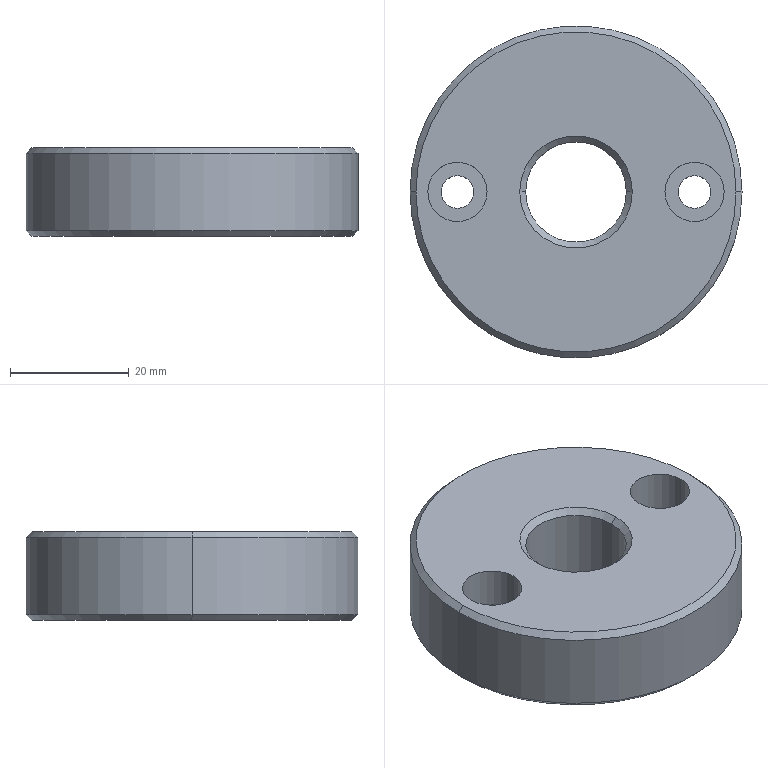Part | SolidWorks | features HoleWzd 2, Chamfer 1, Extrusion 1 | 1 solid | 24 faces | box 56 x 56 x 15 mm | volume 31831 mm3 | cylinder 12 | cone 8 | plane 4 | commonest cylinder face diameters 5.5 x4 10 x4 17 x2 56 x2
STEP:
#1=CARTESIAN_POINT('',(27.,0.,15.));
#2=VERTEX_POINT('',#1);
#3=CARTESIAN_POINT('',(-27.,0.,15.));
#4=VERTEX_POINT('',#3);
#5=CARTESIAN_POINT('',(0.,0.,15.));
#6=DIRECTION('',(0.,0.,1.));
#7=DIRECTION('',(1.,0.,0.));
#8=AXIS2_PLACEMENT_3D('',#5,#6,#7);
#9=CIRCLE('',#8,27.);
#10=EDGE_CURVE('',#2,#4,#9,.T.);
#11=ORIENTED_EDGE('',*,*,#10,.F.);
#12=CARTESIAN_POINT('',(28.,0.,14.));
#13=VERTEX_POINT('',#12);
#14=CARTESIAN_POINT('',(27.,0.,15.));
#15=DIRECTION('',(0.7071,0.,-0.7071));
#16=VECTOR('',#15,1000.);
#17=LINE('',#14,#16);
#18=EDGE_CURVE('',#2,#13,#17,.T.);
#19=ORIENTED_EDGE('',*,*,#18,.T.);
#20=CARTESIAN_POINT('',(-28.,0.,14.));
#21=VERTEX_POINT('',#20);
#22=CARTESIAN_POINT('',(0.,0.,14.));
#23=DIRECTION('',(0.,0.,-1.));
#24=DIRECTION('',(1.,0.,0.));
#25=AXIS2_PLACEMENT_3D('',#22,#23,#24);
#26=CIRCLE('',#25,28.);
#27=EDGE_CURVE('',#21,#13,#26,.T.);
#28=ORIENTED_EDGE('',*,*,#27,.F.);
#29=CARTESIAN_POINT('',(-27.,0.,15.));
#30=DIRECTION('',(-0.7071,0.,-0.7071));
#31=VECTOR('',#30,1000.);
#32=LINE('',#29,#31);
#33=EDGE_CURVE('',#4,#21,#32,.T.);
#34=ORIENTED_EDGE('',*,*,#33,.F.);
#35=EDGE_LOOP('',(#11,#19,#28,#34));
#36=FACE_OUTER_BOUND('',#35,.T.);
#37=CARTESIAN_POINT('',(0.,0.,15.));
#38=DIRECTION('',(0.,0.,-1.));
#39=DIRECTION('',(-1.,0.,0.));
#40=AXIS2_PLACEMENT_3D('',#37,#38,#39);
#41=CONICAL_SURFACE('',#40,27.,0.7854);
#42=ADVANCED_FACE('',(#36),#41,.T.);
#43=CARTESIAN_POINT('',(-27.,0.,0.));
#44=VERTEX_POINT('',#43);
#45=CARTESIAN_POINT('',(27.,0.,0.));
#46=VERTEX_POINT('',#45);
#47=CARTESIAN_POINT('',(0.,0.,0.));
#48=DIRECTION('',(0.,0.,-1.));
#49=DIRECTION('',(1.,0.,0.));
#50=AXIS2_PLACEMENT_3D('',#47,#48,#49);
#51=CIRCLE('',#50,27.);
#52=EDGE_CURVE('',#44,#46,#51,.T.);
#53=ORIENTED_EDGE('',*,*,#52,.F.);
#54=CARTESIAN_POINT('',(-28.,0.,1.));
#55=VERTEX_POINT('',#54);
#56=CARTESIAN_POINT('',(-28.,0.,1.));
#57=DIRECTION('',(-0.7071,0.,0.7071));
#58=VECTOR('',#57,1000.);
#59=LINE('',#56,#58);
#60=EDGE_CURVE('',#44,#55,#59,.T.);
#61=ORIENTED_EDGE('',*,*,#60,.T.);
#62=CARTESIAN_POINT('',(28.,0.,1.));
#63=VERTEX_POINT('',#62);
#64=CARTESIAN_POINT('',(0.,0.,1.));
#65=DIRECTION('',(0.,0.,1.));
#66=DIRECTION('',(1.,0.,0.));
#67=AXIS2_PLACEMENT_3D('',#64,#65,#66);
#68=CIRCLE('',#67,28.);
#69=EDGE_CURVE('',#63,#55,#68,.T.);
#70=ORIENTED_EDGE('',*,*,#69,.F.);
#71=CARTESIAN_POINT('',(28.,0.,1.));
#72=DIRECTION('',(0.7071,0.,0.7071));
#73=VECTOR('',#72,1000.);
#74=LINE('',#71,#73);
#75=EDGE_CURVE('',#46,#63,#74,.T.);
#76=ORIENTED_EDGE('',*,*,#75,.F.);
#77=EDGE_LOOP('',(#53,#61,#70,#76));
#78=FACE_OUTER_BOUND('',#77,.T.);
#79=CARTESIAN_POINT('',(0.,0.,1.));
#80=DIRECTION('',(0.,0.,1.));
#81=DIRECTION('',(1.,0.,0.));
#82=AXIS2_PLACEMENT_3D('',#79,#80,#81);
#83=CONICAL_SURFACE('',#82,28.,0.7854);
#84=ADVANCED_FACE('',(#78),#83,.T.);
#85=CARTESIAN_POINT('',(8.5,0.,1.));
#86=VERTEX_POINT('',#85);
#87=CARTESIAN_POINT('',(-8.5,0.,1.));
#88=VERTEX_POINT('',#87);
#89=CARTESIAN_POINT('',(0.,0.,1.));
#90=DIRECTION('',(0.,0.,-1.));
#91=DIRECTION('',(1.,0.,0.));
#92=AXIS2_PLACEMENT_3D('',#89,#90,#91);
#93=CIRCLE('',#92,8.5);
#94=EDGE_CURVE('',#86,#88,#93,.T.);
#95=ORIENTED_EDGE('',*,*,#94,.F.);
#96=CARTESIAN_POINT('',(9.5,0.,0.));
#97=VERTEX_POINT('',#96);
#98=CARTESIAN_POINT('',(9.5,0.,0.));
#99=DIRECTION('',(0.7071,0.,-0.7071));
#100=VECTOR('',#99,1000.);
#101=LINE('',#98,#100);
#102=EDGE_CURVE('',#86,#97,#101,.T.);
#103=ORIENTED_EDGE('',*,*,#102,.T.);
#104=CARTESIAN_POINT('',(-9.5,0.,0.));
#105=VERTEX_POINT('',#104);
#106=CARTESIAN_POINT('',(0.,0.,0.));
#107=DIRECTION('',(0.,0.,1.));
#108=DIRECTION('',(1.,0.,0.));
#109=AXIS2_PLACEMENT_3D('',#106,#107,#108);
#110=CIRCLE('',#109,9.5);
#111=EDGE_CURVE('',#105,#97,#110,.T.);
#112=ORIENTED_EDGE('',*,*,#111,.F.);
#113=CARTESIAN_POINT('',(-9.5,0.,0.));
#114=DIRECTION('',(-0.7071,0.,-0.7071));
#115=VECTOR('',#114,1000.);
#116=LINE('',#113,#115);
#117=EDGE_CURVE('',#88,#105,#116,.T.);
#118=ORIENTED_EDGE('',*,*,#117,.F.);
#119=EDGE_LOOP('',(#95,#103,#112,#118));
#120=FACE_OUTER_BOUND('',#119,.T.);
#121=CARTESIAN_POINT('',(0.,0.,0.));
#122=DIRECTION('',(0.,0.,-1.));
#123=DIRECTION('',(-1.,0.,0.));
#124=AXIS2_PLACEMENT_3D('',#121,#122,#123);
#125=CONICAL_SURFACE('',#124,9.5,0.7854);
#126=ADVANCED_FACE('',(#120),#125,.F.);
#127=CARTESIAN_POINT('',(-8.5,0.,14.));
#128=VERTEX_POINT('',#127);
#129=CARTESIAN_POINT('',(8.5,0.,14.));
#130=VERTEX_POINT('',#129);
#131=CARTESIAN_POINT('',(0.,0.,14.));
#132=DIRECTION('',(0.,0.,1.));
#133=DIRECTION('',(1.,0.,0.));
#134=AXIS2_PLACEMENT_3D('',#131,#132,#133);
#135=CIRCLE('',#134,8.5);
#136=EDGE_CURVE('',#128,#130,#135,.T.);
#137=ORIENTED_EDGE('',*,*,#136,.F.);
#138=CARTESIAN_POINT('',(-9.5,0.,15.));
#139=VERTEX_POINT('',#138);
#140=CARTESIAN_POINT('',(-8.5,0.,14.));
#141=DIRECTION('',(-0.7071,0.,0.7071));
#142=VECTOR('',#141,1000.);
#143=LINE('',#140,#142);
#144=EDGE_CURVE('',#128,#139,#143,.T.);
#145=ORIENTED_EDGE('',*,*,#144,.T.);
#146=CARTESIAN_POINT('',(9.5,0.,15.));
#147=VERTEX_POINT('',#146);
#148=CARTESIAN_POINT('',(0.,0.,15.));
#149=DIRECTION('',(0.,0.,-1.));
#150=DIRECTION('',(1.,0.,0.));
#151=AXIS2_PLACEMENT_3D('',#148,#149,#150);
#152=CIRCLE('',#151,9.5);
#153=EDGE_CURVE('',#147,#139,#152,.T.);
#154=ORIENTED_EDGE('',*,*,#153,.F.);
#155=CARTESIAN_POINT('',(8.5,0.,14.));
#156=DIRECTION('',(0.7071,0.,0.7071));
#157=VECTOR('',#156,1000.);
#158=LINE('',#155,#157);
#159=EDGE_CURVE('',#130,#147,#158,.T.);
#160=ORIENTED_EDGE('',*,*,#159,.F.);
#161=EDGE_LOOP('',(#137,#145,#154,#160));
#162=FACE_OUTER_BOUND('',#161,.T.);
#163=CARTESIAN_POINT('',(0.,0.,14.));
#164=DIRECTION('',(0.,0.,1.));
#165=DIRECTION('',(1.,0.,0.));
#166=AXIS2_PLACEMENT_3D('',#163,#164,#165);
#167=CONICAL_SURFACE('',#166,8.5,0.7854);
#168=ADVANCED_FACE('',(#162),#167,.F.);
#169=CARTESIAN_POINT('',(-25.,0.,8.));
#170=VERTEX_POINT('',#169);
#171=CARTESIAN_POINT('',(-15.,0.,8.));
#172=VERTEX_POINT('',#171);
#173=CARTESIAN_POINT('',(-20.,0.,8.));
#174=DIRECTION('',(0.,0.,1.));
#175=DIRECTION('',(1.,0.,0.));
#176=AXIS2_PLACEMENT_3D('',#173,#174,#175);
#177=CIRCLE('',#176,5.);
#178=EDGE_CURVE('',#170,#172,#177,.T.);
#179=ORIENTED_EDGE('',*,*,#178,.F.);
#180=CARTESIAN_POINT('',(-25.,0.,15.));
#181=VERTEX_POINT('',#180);
#182=CARTESIAN_POINT('',(-25.,0.,15.));
#183=DIRECTION('',(0.,0.,1.));
#184=VECTOR('',#183,1000.);
#185=LINE('',#182,#184);
#186=EDGE_CURVE('',#170,#181,#185,.T.);
#187=ORIENTED_EDGE('',*,*,#186,.T.);
#188=CARTESIAN_POINT('',(-15.,0.,15.));
#189=VERTEX_POINT('',#188);
#190=CARTESIAN_POINT('',(-20.,0.,15.));
#191=DIRECTION('',(0.,0.,1.));
#192=DIRECTION('',(1.,0.,0.));
#193=AXIS2_PLACEMENT_3D('',#190,#191,#192);
#194=CIRCLE('',#193,5.);
#195=EDGE_CURVE('',#181,#189,#194,.T.);
#196=ORIENTED_EDGE('',*,*,#195,.T.);
#197=CARTESIAN_POINT('',(-15.,0.,15.));
#198=DIRECTION('',(0.,0.,1.));
#199=VECTOR('',#198,1000.);
#200=LINE('',#197,#199);
#201=EDGE_CURVE('',#172,#189,#200,.T.);
#202=ORIENTED_EDGE('',*,*,#201,.F.);
#203=EDGE_LOOP('',(#179,#187,#196,#202));
#204=FACE_OUTER_BOUND('',#203,.T.);
#205=CARTESIAN_POINT('',(-20.,0.,15.));
#206=DIRECTION('',(0.,0.,1.));
#207=DIRECTION('',(1.,0.,0.));
#208=AXIS2_PLACEMENT_3D('',#205,#206,#207);
#209=CYLINDRICAL_SURFACE('',#208,5.);
#210=ADVANCED_FACE('',(#204),#209,.F.);
#211=CARTESIAN_POINT('',(-22.75,0.,0.));
#212=VERTEX_POINT('',#211);
#213=CARTESIAN_POINT('',(-17.25,0.,0.));
#214=VERTEX_POINT('',#213);
#215=CARTESIAN_POINT('',(-20.,0.,0.));
#216=DIRECTION('',(0.,0.,1.));
#217=DIRECTION('',(1.,0.,0.));
#218=AXIS2_PLACEMENT_3D('',#215,#216,#217);
#219=CIRCLE('',#218,2.75);
#220=EDGE_CURVE('',#212,#214,#219,.T.);
#221=ORIENTED_EDGE('',*,*,#220,.F.);
#222=CARTESIAN_POINT('',(-22.75,0.,8.));
#223=VERTEX_POINT('',#222);
#224=CARTESIAN_POINT('',(-22.75,0.,15.));
#225=DIRECTION('',(0.,0.,1.));
#226=VECTOR('',#225,1000.);
#227=LINE('',#224,#226);
#228=EDGE_CURVE('',#212,#223,#227,.T.);
#229=ORIENTED_EDGE('',*,*,#228,.T.);
#230=CARTESIAN_POINT('',(-17.25,0.,8.));
#231=VERTEX_POINT('',#230);
#232=CARTESIAN_POINT('',(-20.,0.,8.));
#233=DIRECTION('',(0.,0.,1.));
#234=DIRECTION('',(1.,0.,0.));
#235=AXIS2_PLACEMENT_3D('',#232,#233,#234);
#236=CIRCLE('',#235,2.75);
#237=EDGE_CURVE('',#223,#231,#236,.T.);
#238=ORIENTED_EDGE('',*,*,#237,.T.);
#239=CARTESIAN_POINT('',(-17.25,0.,15.));
#240=DIRECTION('',(0.,0.,1.));
#241=VECTOR('',#240,1000.);
#242=LINE('',#239,#241);
#243=EDGE_CURVE('',#214,#231,#242,.T.);
#244=ORIENTED_EDGE('',*,*,#243,.F.);
#245=EDGE_LOOP('',(#221,#229,#238,#244));
#246=FACE_OUTER_BOUND('',#245,.T.);
#247=CARTESIAN_POINT('',(-20.,0.,15.));
#248=DIRECTION('',(0.,0.,1.));
#249=DIRECTION('',(1.,0.,0.));
#250=AXIS2_PLACEMENT_3D('',#247,#248,#249);
#251=CYLINDRICAL_SURFACE('',#250,2.75);
#252=ADVANCED_FACE('',(#246),#251,.F.);
#253=CARTESIAN_POINT('',(15.,0.,8.));
#254=VERTEX_POINT('',#253);
#255=CARTESIAN_POINT('',(25.,0.,8.));
#256=VERTEX_POINT('',#255);
#257=CARTESIAN_POINT('',(20.,0.,8.));
#258=DIRECTION('',(0.,0.,1.));
#259=DIRECTION('',(1.,0.,0.));
#260=AXIS2_PLACEMENT_3D('',#257,#258,#259);
#261=CIRCLE('',#260,5.);
#262=EDGE_CURVE('',#254,#256,#261,.T.);
#263=ORIENTED_EDGE('',*,*,#262,.F.);
#264=CARTESIAN_POINT('',(15.,0.,15.));
#265=VERTEX_POINT('',#264);
#266=CARTESIAN_POINT('',(15.,0.,15.));
#267=DIRECTION('',(0.,0.,1.));
#268=VECTOR('',#267,1000.);
#269=LINE('',#266,#268);
#270=EDGE_CURVE('',#254,#265,#269,.T.);
#271=ORIENTED_EDGE('',*,*,#270,.T.);
#272=CARTESIAN_POINT('',(25.,0.,15.));
#273=VERTEX_POINT('',#272);
#274=CARTESIAN_POINT('',(20.,0.,15.));
#275=DIRECTION('',(0.,0.,1.));
#276=DIRECTION('',(1.,0.,0.));
#277=AXIS2_PLACEMENT_3D('',#274,#275,#276);
#278=CIRCLE('',#277,5.);
#279=EDGE_CURVE('',#265,#273,#278,.T.);
#280=ORIENTED_EDGE('',*,*,#279,.T.);
#281=CARTESIAN_POINT('',(25.,0.,15.));
#282=DIRECTION('',(0.,0.,1.));
#283=VECTOR('',#282,1000.);
#284=LINE('',#281,#283);
#285=EDGE_CURVE('',#256,#273,#284,.T.);
#286=ORIENTED_EDGE('',*,*,#285,.F.);
#287=EDGE_LOOP('',(#263,#271,#280,#286));
#288=FACE_OUTER_BOUND('',#287,.T.);
#289=CARTESIAN_POINT('',(20.,0.,15.));
#290=DIRECTION('',(0.,0.,1.));
#291=DIRECTION('',(1.,0.,0.));
#292=AXIS2_PLACEMENT_3D('',#289,#290,#291);
#293=CYLINDRICAL_SURFACE('',#292,5.);
#294=ADVANCED_FACE('',(#288),#293,.F.);
#295=CARTESIAN_POINT('',(17.25,0.,0.));
#296=VERTEX_POINT('',#295);
#297=CARTESIAN_POINT('',(22.75,0.,0.));
#298=VERTEX_POINT('',#297);
#299=CARTESIAN_POINT('',(20.,0.,0.));
#300=DIRECTION('',(0.,0.,1.));
#301=DIRECTION('',(1.,0.,0.));
#302=AXIS2_PLACEMENT_3D('',#299,#300,#301);
#303=CIRCLE('',#302,2.75);
#304=EDGE_CURVE('',#296,#298,#303,.T.);
#305=ORIENTED_EDGE('',*,*,#304,.F.);
#306=CARTESIAN_POINT('',(17.25,0.,8.));
#307=VERTEX_POINT('',#306);
#308=CARTESIAN_POINT('',(17.25,0.,15.));
#309=DIRECTION('',(0.,0.,1.));
#310=VECTOR('',#309,1000.);
#311=LINE('',#308,#310);
#312=EDGE_CURVE('',#296,#307,#311,.T.);
#313=ORIENTED_EDGE('',*,*,#312,.T.);
#314=CARTESIAN_POINT('',(22.75,0.,8.));
#315=VERTEX_POINT('',#314);
#316=CARTESIAN_POINT('',(20.,0.,8.));
#317=DIRECTION('',(0.,0.,1.));
#318=DIRECTION('',(1.,0.,0.));
#319=AXIS2_PLACEMENT_3D('',#316,#317,#318);
#320=CIRCLE('',#319,2.75);
#321=EDGE_CURVE('',#307,#315,#320,.T.);
#322=ORIENTED_EDGE('',*,*,#321,.T.);
#323=CARTESIAN_POINT('',(22.75,0.,15.));
#324=DIRECTION('',(0.,0.,1.));
#325=VECTOR('',#324,1000.);
#326=LINE('',#323,#325);
#327=EDGE_CURVE('',#298,#315,#326,.T.);
#328=ORIENTED_EDGE('',*,*,#327,.F.);
#329=EDGE_LOOP('',(#305,#313,#322,#328));
#330=FACE_OUTER_BOUND('',#329,.T.);
#331=CARTESIAN_POINT('',(20.,0.,15.));
#332=DIRECTION('',(0.,0.,1.));
#333=DIRECTION('',(1.,0.,0.));
#334=AXIS2_PLACEMENT_3D('',#331,#332,#333);
#335=CYLINDRICAL_SURFACE('',#334,2.75);
#336=ADVANCED_FACE('',(#330),#335,.F.);
#337=ORIENTED_EDGE('',*,*,#94,.T.);
#338=CARTESIAN_POINT('',(-8.5,0.,15.));
#339=DIRECTION('',(0.,0.,1.));
#340=VECTOR('',#339,1000.);
#341=LINE('',#338,#340);
#342=EDGE_CURVE('',#88,#128,#341,.T.);
#343=ORIENTED_EDGE('',*,*,#342,.T.);
#344=ORIENTED_EDGE('',*,*,#136,.T.);
#345=CARTESIAN_POINT('',(8.5,0.,15.));
#346=DIRECTION('',(0.,0.,1.));
#347=VECTOR('',#346,1000.);
#348=LINE('',#345,#347);
#349=EDGE_CURVE('',#86,#130,#348,.T.);
#350=ORIENTED_EDGE('',*,*,#349,.F.);
#351=EDGE_LOOP('',(#337,#343,#344,#350));
#352=FACE_OUTER_BOUND('',#351,.T.);
#353=CARTESIAN_POINT('',(0.,0.,15.));
#354=DIRECTION('',(0.,0.,1.));
#355=DIRECTION('',(1.,0.,0.));
#356=AXIS2_PLACEMENT_3D('',#353,#354,#355);
#357=CYLINDRICAL_SURFACE('',#356,8.5);
#358=ADVANCED_FACE('',(#352),#357,.F.);
#359=ORIENTED_EDGE('',*,*,#27,.T.);
#360=CARTESIAN_POINT('',(28.,0.,15.));
#361=DIRECTION('',(0.,0.,-1.));
#362=VECTOR('',#361,1000.);
#363=LINE('',#360,#362);
#364=EDGE_CURVE('',#13,#63,#363,.T.);
#365=ORIENTED_EDGE('',*,*,#364,.T.);
#366=ORIENTED_EDGE('',*,*,#69,.T.);
#367=CARTESIAN_POINT('',(-28.,0.,15.));
#368=DIRECTION('',(0.,0.,-1.));
#369=VECTOR('',#368,1000.);
#370=LINE('',#367,#369);
#371=EDGE_CURVE('',#21,#55,#370,.T.);
#372=ORIENTED_EDGE('',*,*,#371,.F.);
#373=EDGE_LOOP('',(#359,#365,#366,#372));
#374=FACE_OUTER_BOUND('',#373,.T.);
#375=CARTESIAN_POINT('',(0.,0.,15.));
#376=DIRECTION('',(0.,0.,-1.));
#377=DIRECTION('',(-1.,0.,0.));
#378=AXIS2_PLACEMENT_3D('',#375,#376,#377);
#379=CYLINDRICAL_SURFACE('',#378,28.);
#380=ADVANCED_FACE('',(#374),#379,.T.);
#381=ORIENTED_EDGE('',*,*,#364,.F.);
#382=CARTESIAN_POINT('',(0.,0.,14.));
#383=DIRECTION('',(0.,0.,-1.));
#384=DIRECTION('',(1.,0.,0.));
#385=AXIS2_PLACEMENT_3D('',#382,#383,#384);
#386=CIRCLE('',#385,28.);
#387=EDGE_CURVE('',#13,#21,#386,.T.);
#388=ORIENTED_EDGE('',*,*,#387,.T.);
#389=ORIENTED_EDGE('',*,*,#371,.T.);
#390=CARTESIAN_POINT('',(0.,0.,1.));
#391=DIRECTION('',(0.,0.,1.));
#392=DIRECTION('',(1.,0.,0.));
#393=AXIS2_PLACEMENT_3D('',#390,#391,#392);
#394=CIRCLE('',#393,28.);
#395=EDGE_CURVE('',#55,#63,#394,.T.);
#396=ORIENTED_EDGE('',*,*,#395,.T.);
#397=EDGE_LOOP('',(#381,#388,#389,#396));
#398=FACE_OUTER_BOUND('',#397,.T.);
#399=CARTESIAN_POINT('',(0.,0.,15.));
#400=DIRECTION('',(0.,0.,-1.));
#401=DIRECTION('',(-1.,0.,0.));
#402=AXIS2_PLACEMENT_3D('',#399,#400,#401);
#403=CYLINDRICAL_SURFACE('',#402,28.);
#404=ADVANCED_FACE('',(#398),#403,.T.);
#405=ORIENTED_EDGE('',*,*,#153,.T.);
#406=CARTESIAN_POINT('',(0.,0.,15.));
#407=DIRECTION('',(0.,0.,-1.));
#408=DIRECTION('',(1.,0.,0.));
#409=AXIS2_PLACEMENT_3D('',#406,#407,#408);
#410=CIRCLE('',#409,9.5);
#411=EDGE_CURVE('',#139,#147,#410,.T.);
#412=ORIENTED_EDGE('',*,*,#411,.T.);
#413=EDGE_LOOP('',(#405,#412));
#414=FACE_BOUND('',#413,.T.);
#415=CARTESIAN_POINT('',(0.,0.,15.));
#416=DIRECTION('',(0.,0.,1.));
#417=DIRECTION('',(1.,0.,0.));
#418=AXIS2_PLACEMENT_3D('',#415,#416,#417);
#419=CIRCLE('',#418,27.);
#420=EDGE_CURVE('',#4,#2,#419,.T.);
#421=ORIENTED_EDGE('',*,*,#420,.T.);
#422=ORIENTED_EDGE('',*,*,#10,.T.);
#423=EDGE_LOOP('',(#421,#422));
#424=FACE_OUTER_BOUND('',#423,.T.);
#425=CARTESIAN_POINT('',(-20.,0.,15.));
#426=DIRECTION('',(0.,0.,1.));
#427=DIRECTION('',(1.,0.,0.));
#428=AXIS2_PLACEMENT_3D('',#425,#426,#427);
#429=CIRCLE('',#428,5.);
#430=EDGE_CURVE('',#189,#181,#429,.T.);
#431=ORIENTED_EDGE('',*,*,#430,.F.);
#432=ORIENTED_EDGE('',*,*,#195,.F.);
#433=EDGE_LOOP('',(#431,#432));
#434=FACE_BOUND('',#433,.T.);
#435=CARTESIAN_POINT('',(20.,0.,15.));
#436=DIRECTION('',(0.,0.,1.));
#437=DIRECTION('',(1.,0.,0.));
#438=AXIS2_PLACEMENT_3D('',#435,#436,#437);
#439=CIRCLE('',#438,5.);
#440=EDGE_CURVE('',#273,#265,#439,.T.);
#441=ORIENTED_EDGE('',*,*,#440,.F.);
#442=ORIENTED_EDGE('',*,*,#279,.F.);
#443=EDGE_LOOP('',(#441,#442));
#444=FACE_BOUND('',#443,.T.);
#445=CARTESIAN_POINT('',(0.,0.,15.));
#446=DIRECTION('',(0.,0.,1.));
#447=DIRECTION('',(1.,0.,0.));
#448=AXIS2_PLACEMENT_3D('',#445,#446,#447);
#449=PLANE('',#448);
#450=ADVANCED_FACE('',(#414,#424,#434,#444),#449,.T.);
#451=ORIENTED_EDGE('',*,*,#111,.T.);
#452=CARTESIAN_POINT('',(0.,0.,0.));
#453=DIRECTION('',(0.,0.,1.));
#454=DIRECTION('',(1.,0.,0.));
#455=AXIS2_PLACEMENT_3D('',#452,#453,#454);
#456=CIRCLE('',#455,9.5);
#457=EDGE_CURVE('',#97,#105,#456,.T.);
#458=ORIENTED_EDGE('',*,*,#457,.T.);
#459=EDGE_LOOP('',(#451,#458));
#460=FACE_BOUND('',#459,.T.);
#461=CARTESIAN_POINT('',(0.,0.,0.));
#462=DIRECTION('',(0.,0.,-1.));
#463=DIRECTION('',(1.,0.,0.));
#464=AXIS2_PLACEMENT_3D('',#461,#462,#463);
#465=CIRCLE('',#464,27.);
#466=EDGE_CURVE('',#46,#44,#465,.T.);
#467=ORIENTED_EDGE('',*,*,#466,.T.);
#468=ORIENTED_EDGE('',*,*,#52,.T.);
#469=EDGE_LOOP('',(#467,#468));
#470=FACE_OUTER_BOUND('',#469,.T.);
#471=CARTESIAN_POINT('',(-20.,0.,0.));
#472=DIRECTION('',(0.,0.,1.));
#473=DIRECTION('',(1.,0.,0.));
#474=AXIS2_PLACEMENT_3D('',#471,#472,#473);
#475=CIRCLE('',#474,2.75);
#476=EDGE_CURVE('',#214,#212,#475,.T.);
#477=ORIENTED_EDGE('',*,*,#476,.T.);
#478=ORIENTED_EDGE('',*,*,#220,.T.);
#479=EDGE_LOOP('',(#477,#478));
#480=FACE_BOUND('',#479,.T.);
#481=CARTESIAN_POINT('',(20.,0.,0.));
#482=DIRECTION('',(0.,0.,1.));
#483=DIRECTION('',(1.,0.,0.));
#484=AXIS2_PLACEMENT_3D('',#481,#482,#483);
#485=CIRCLE('',#484,2.75);
#486=EDGE_CURVE('',#298,#296,#485,.T.);
#487=ORIENTED_EDGE('',*,*,#486,.T.);
#488=ORIENTED_EDGE('',*,*,#304,.T.);
#489=EDGE_LOOP('',(#487,#488));
#490=FACE_BOUND('',#489,.T.);
#491=CARTESIAN_POINT('',(0.,0.,0.));
#492=DIRECTION('',(0.,0.,1.));
#493=DIRECTION('',(1.,0.,0.));
#494=AXIS2_PLACEMENT_3D('',#491,#492,#493);
#495=PLANE('',#494);
#496=ADVANCED_FACE('',(#460,#470,#480,#490),#495,.F.);
#497=ORIENTED_EDGE('',*,*,#342,.F.);
#498=CARTESIAN_POINT('',(0.,0.,1.));
#499=DIRECTION('',(0.,0.,-1.));
#500=DIRECTION('',(1.,0.,0.));
#501=AXIS2_PLACEMENT_3D('',#498,#499,#500);
#502=CIRCLE('',#501,8.5);
#503=EDGE_CURVE('',#88,#86,#502,.T.);
#504=ORIENTED_EDGE('',*,*,#503,.T.);
#505=ORIENTED_EDGE('',*,*,#349,.T.);
#506=CARTESIAN_POINT('',(0.,0.,14.));
#507=DIRECTION('',(0.,0.,1.));
#508=DIRECTION('',(1.,0.,0.));
#509=AXIS2_PLACEMENT_3D('',#506,#507,#508);
#510=CIRCLE('',#509,8.5);
#511=EDGE_CURVE('',#130,#128,#510,.T.);
#512=ORIENTED_EDGE('',*,*,#511,.T.);
#513=EDGE_LOOP('',(#497,#504,#505,#512));
#514=FACE_OUTER_BOUND('',#513,.T.);
#515=CARTESIAN_POINT('',(0.,0.,15.));
#516=DIRECTION('',(0.,0.,1.));
#517=DIRECTION('',(1.,0.,0.));
#518=AXIS2_PLACEMENT_3D('',#515,#516,#517);
#519=CYLINDRICAL_SURFACE('',#518,8.5);
#520=ADVANCED_FACE('',(#514),#519,.F.);
#521=ORIENTED_EDGE('',*,*,#312,.F.);
#522=ORIENTED_EDGE('',*,*,#486,.F.);
#523=ORIENTED_EDGE('',*,*,#327,.T.);
#524=CARTESIAN_POINT('',(20.,0.,8.));
#525=DIRECTION('',(0.,0.,1.));
#526=DIRECTION('',(1.,0.,0.));
#527=AXIS2_PLACEMENT_3D('',#524,#525,#526);
#528=CIRCLE('',#527,2.75);
#529=EDGE_CURVE('',#315,#307,#528,.T.);
#530=ORIENTED_EDGE('',*,*,#529,.T.);
#531=EDGE_LOOP('',(#521,#522,#523,#530));
#532=FACE_OUTER_BOUND('',#531,.T.);
#533=CARTESIAN_POINT('',(20.,0.,15.));
#534=DIRECTION('',(0.,0.,1.));
#535=DIRECTION('',(1.,0.,0.));
#536=AXIS2_PLACEMENT_3D('',#533,#534,#535);
#537=CYLINDRICAL_SURFACE('',#536,2.75);
#538=ADVANCED_FACE('',(#532),#537,.F.);
#539=ORIENTED_EDGE('',*,*,#529,.F.);
#540=ORIENTED_EDGE('',*,*,#321,.F.);
#541=EDGE_LOOP('',(#539,#540));
#542=FACE_BOUND('',#541,.T.);
#543=CARTESIAN_POINT('',(20.,0.,8.));
#544=DIRECTION('',(0.,0.,1.));
#545=DIRECTION('',(1.,0.,0.));
#546=AXIS2_PLACEMENT_3D('',#543,#544,#545);
#547=CIRCLE('',#546,5.);
#548=EDGE_CURVE('',#256,#254,#547,.T.);
#549=ORIENTED_EDGE('',*,*,#548,.T.);
#550=ORIENTED_EDGE('',*,*,#262,.T.);
#551=EDGE_LOOP('',(#549,#550));
#552=FACE_OUTER_BOUND('',#551,.T.);
#553=CARTESIAN_POINT('',(22.75,0.,8.));
#554=DIRECTION('',(0.,0.,-1.));
#555=DIRECTION('',(-1.,0.,0.));
#556=AXIS2_PLACEMENT_3D('',#553,#554,#555);
#557=PLANE('',#556);
#558=ADVANCED_FACE('',(#542,#552),#557,.F.);
#559=ORIENTED_EDGE('',*,*,#270,.F.);
#560=ORIENTED_EDGE('',*,*,#548,.F.);
#561=ORIENTED_EDGE('',*,*,#285,.T.);
#562=ORIENTED_EDGE('',*,*,#440,.T.);
#563=EDGE_LOOP('',(#559,#560,#561,#562));
#564=FACE_OUTER_BOUND('',#563,.T.);
#565=CARTESIAN_POINT('',(20.,0.,15.));
#566=DIRECTION('',(0.,0.,1.));
#567=DIRECTION('',(1.,0.,0.));
#568=AXIS2_PLACEMENT_3D('',#565,#566,#567);
#569=CYLINDRICAL_SURFACE('',#568,5.);
#570=ADVANCED_FACE('',(#564),#569,.F.);
#571=ORIENTED_EDGE('',*,*,#228,.F.);
#572=ORIENTED_EDGE('',*,*,#476,.F.);
#573=ORIENTED_EDGE('',*,*,#243,.T.);
#574=CARTESIAN_POINT('',(-20.,0.,8.));
#575=DIRECTION('',(0.,0.,1.));
#576=DIRECTION('',(1.,0.,0.));
#577=AXIS2_PLACEMENT_3D('',#574,#575,#576);
#578=CIRCLE('',#577,2.75);
#579=EDGE_CURVE('',#231,#223,#578,.T.);
#580=ORIENTED_EDGE('',*,*,#579,.T.);
#581=EDGE_LOOP('',(#571,#572,#573,#580));
#582=FACE_OUTER_BOUND('',#581,.T.);
#583=CARTESIAN_POINT('',(-20.,0.,15.));
#584=DIRECTION('',(0.,0.,1.));
#585=DIRECTION('',(1.,0.,0.));
#586=AXIS2_PLACEMENT_3D('',#583,#584,#585);
#587=CYLINDRICAL_SURFACE('',#586,2.75);
#588=ADVANCED_FACE('',(#582),#587,.F.);
#589=ORIENTED_EDGE('',*,*,#579,.F.);
#590=ORIENTED_EDGE('',*,*,#237,.F.);
#591=EDGE_LOOP('',(#589,#590));
#592=FACE_BOUND('',#591,.T.);
#593=CARTESIAN_POINT('',(-20.,0.,8.));
#594=DIRECTION('',(0.,0.,1.));
#595=DIRECTION('',(1.,0.,0.));
#596=AXIS2_PLACEMENT_3D('',#593,#594,#595);
#597=CIRCLE('',#596,5.);
#598=EDGE_CURVE('',#172,#170,#597,.T.);
#599=ORIENTED_EDGE('',*,*,#598,.T.);
#600=ORIENTED_EDGE('',*,*,#178,.T.);
#601=EDGE_LOOP('',(#599,#600));
#602=FACE_OUTER_BOUND('',#601,.T.);
#603=CARTESIAN_POINT('',(-17.25,0.,8.));
#604=DIRECTION('',(0.,0.,-1.));
#605=DIRECTION('',(-1.,0.,0.));
#606=AXIS2_PLACEMENT_3D('',#603,#604,#605);
#607=PLANE('',#606);
#608=ADVANCED_FACE('',(#592,#602),#607,.F.);
#609=ORIENTED_EDGE('',*,*,#186,.F.);
#610=ORIENTED_EDGE('',*,*,#598,.F.);
#611=ORIENTED_EDGE('',*,*,#201,.T.);
#612=ORIENTED_EDGE('',*,*,#430,.T.);
#613=EDGE_LOOP('',(#609,#610,#611,#612));
#614=FACE_OUTER_BOUND('',#613,.T.);
#615=CARTESIAN_POINT('',(-20.,0.,15.));
#616=DIRECTION('',(0.,0.,1.));
#617=DIRECTION('',(1.,0.,0.));
#618=AXIS2_PLACEMENT_3D('',#615,#616,#617);
#619=CYLINDRICAL_SURFACE('',#618,5.);
#620=ADVANCED_FACE('',(#614),#619,.F.);
#621=ORIENTED_EDGE('',*,*,#144,.F.);
#622=ORIENTED_EDGE('',*,*,#511,.F.);
#623=ORIENTED_EDGE('',*,*,#159,.T.);
#624=ORIENTED_EDGE('',*,*,#411,.F.);
#625=EDGE_LOOP('',(#621,#622,#623,#624));
#626=FACE_OUTER_BOUND('',#625,.T.);
#627=CARTESIAN_POINT('',(0.,0.,14.));
#628=DIRECTION('',(0.,0.,1.));
#629=DIRECTION('',(1.,0.,0.));
#630=AXIS2_PLACEMENT_3D('',#627,#628,#629);
#631=CONICAL_SURFACE('',#630,8.5,0.7854);
#632=ADVANCED_FACE('',(#626),#631,.F.);
#633=ORIENTED_EDGE('',*,*,#102,.F.);
#634=ORIENTED_EDGE('',*,*,#503,.F.);
#635=ORIENTED_EDGE('',*,*,#117,.T.);
#636=ORIENTED_EDGE('',*,*,#457,.F.);
#637=EDGE_LOOP('',(#633,#634,#635,#636));
#638=FACE_OUTER_BOUND('',#637,.T.);
#639=CARTESIAN_POINT('',(0.,0.,0.));
#640=DIRECTION('',(0.,0.,-1.));
#641=DIRECTION('',(-1.,0.,0.));
#642=AXIS2_PLACEMENT_3D('',#639,#640,#641);
#643=CONICAL_SURFACE('',#642,9.5,0.7854);
#644=ADVANCED_FACE('',(#638),#643,.F.);
#645=ORIENTED_EDGE('',*,*,#60,.F.);
#646=ORIENTED_EDGE('',*,*,#466,.F.);
#647=ORIENTED_EDGE('',*,*,#75,.T.);
#648=ORIENTED_EDGE('',*,*,#395,.F.);
#649=EDGE_LOOP('',(#645,#646,#647,#648));
#650=FACE_OUTER_BOUND('',#649,.T.);
#651=CARTESIAN_POINT('',(0.,0.,1.));
#652=DIRECTION('',(0.,0.,1.));
#653=DIRECTION('',(1.,0.,0.));
#654=AXIS2_PLACEMENT_3D('',#651,#652,#653);
#655=CONICAL_SURFACE('',#654,28.,0.7854);
#656=ADVANCED_FACE('',(#650),#655,.T.);
#657=ORIENTED_EDGE('',*,*,#18,.F.);
#658=ORIENTED_EDGE('',*,*,#420,.F.);
#659=ORIENTED_EDGE('',*,*,#33,.T.);
#660=ORIENTED_EDGE('',*,*,#387,.F.);
#661=EDGE_LOOP('',(#657,#658,#659,#660));
#662=FACE_OUTER_BOUND('',#661,.T.);
#663=CARTESIAN_POINT('',(0.,0.,15.));
#664=DIRECTION('',(0.,0.,-1.));
#665=DIRECTION('',(-1.,0.,0.));
#666=AXIS2_PLACEMENT_3D('',#663,#664,#665);
#667=CONICAL_SURFACE('',#666,27.,0.7854);
#668=ADVANCED_FACE('',(#662),#667,.T.);
#669=CLOSED_SHELL('',(#42,#84,#126,#168,#210,#252,#294,#336,#358,#380,#404,#450,#496,#520,#538,#558,#570,#588,#608,#620,#632,#644,#656,#668));
#670=MANIFOLD_SOLID_BREP('',#669);
#671=CARTESIAN_POINT('',(0.,0.,0.));
#672=DIRECTION('',(0.,0.,1.));
#673=DIRECTION('',(1.,0.,0.));
#674=AXIS2_PLACEMENT_3D('',#671,#672,#673);
#675=(LENGTH_UNIT()NAMED_UNIT(*)SI_UNIT(.MILLI.,.METRE.));
#676=UNCERTAINTY_MEASURE_WITH_UNIT(LENGTH_MEASURE(0.00001),#675,'','');
#677=(NAMED_UNIT(*)PLANE_ANGLE_UNIT()SI_UNIT($,.RADIAN.));
#678=(NAMED_UNIT(*)SI_UNIT($,.STERADIAN.)SOLID_ANGLE_UNIT());
#679=(GEOMETRIC_REPRESENTATION_CONTEXT(3)GLOBAL_UNCERTAINTY_ASSIGNED_CONTEXT((#676))GLOBAL_UNIT_ASSIGNED_CONTEXT((#675,#677,#678))REPRESENTATION_CONTEXT('',''));
#680=ADVANCED_BREP_SHAPE_REPRESENTATION('',(#670,#674),#679);